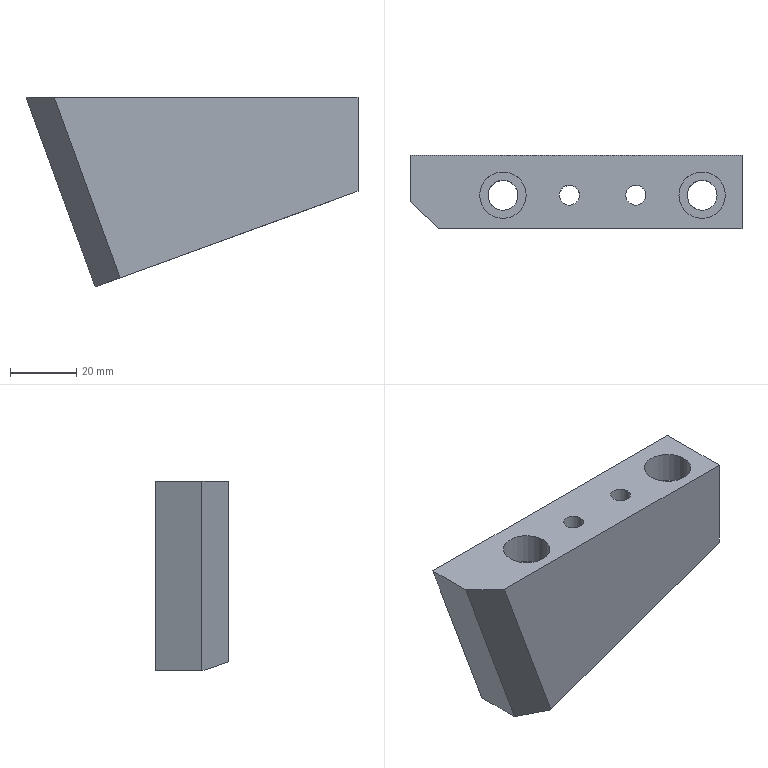Part | STEP file | P011002S003-005 | 1 solid | 15 faces | box 100 x 22 x 57.18 mm | volume 75947 mm3 | plane 9 | cylinder 6 | commonest cylinder face diameters 6 x2 9 x2 14 x2
STEP:
#1=CARTESIAN_POINT('',(0.,0.,0.));
#2=DIRECTION('',(0.,0.,1.));
#3=DIRECTION('',(1.,0.,0.));
#4=AXIS2_PLACEMENT_3D('',#1,#2,#3);
#5=CARTESIAN_POINT('',(-244.,-131.,19.));
#6=VERTEX_POINT('',#5);
#7=CARTESIAN_POINT('',(-237.,-131.,19.));
#8=DIRECTION('',(0.,0.,-1.));
#9=DIRECTION('',(-1.,0.,0.));
#10=AXIS2_PLACEMENT_3D('',#7,#8,#9);
#11=CIRCLE('',#10,7.);
#12=CARTESIAN_POINT('',(-275.,-325.,19.));
#13=DIRECTION('',(0.,0.,1.));
#14=DIRECTION('',(-1.,0.,0.));
#15=AXIS2_PLACEMENT_3D('',#12,#13,#14);
#16=PLANE('',#15);
#17=CARTESIAN_POINT('',(-31.,-194.));
#18=CARTESIAN_POINT('',(-31.,-206.124));
#19=CARTESIAN_POINT('',(-41.5,-200.062));
#20=CARTESIAN_POINT('',(-52.,-194.));
#21=CARTESIAN_POINT('',(-41.5,-187.938));
#22=CARTESIAN_POINT('',(-31.,-181.876));
#23=CARTESIAN_POINT('',(-31.,-194.));
#24=(BOUNDED_CURVE()B_SPLINE_CURVE(2,(#17,#18,#19,#20,#21,#22,#23),.UNSPECIFIED.,.T.,.F.)B_SPLINE_CURVE_WITH_KNOTS((1,2,2,2,2,1),(-2.094,0.,2.094,4.189,6.283,8.378),.UNSPECIFIED.)CURVE()GEOMETRIC_REPRESENTATION_ITEM()RATIONAL_B_SPLINE_CURVE((1.,0.5,1.,0.5,1.,0.5,1.))REPRESENTATION_ITEM(''));
#25=(GEOMETRIC_REPRESENTATION_CONTEXT(2)PARAMETRIC_REPRESENTATION_CONTEXT()REPRESENTATION_CONTEXT('',''));
#26=DEFINITIONAL_REPRESENTATION('',(#24),#25);
#27=PCURVE('',#16,#26);
#28=CARTESIAN_POINT('',(-237.,-131.,19.));
#29=DIRECTION('',(0.,0.,-1.));
#30=DIRECTION('',(1.,0.,0.));
#31=AXIS2_PLACEMENT_3D('',#28,#29,#30);
#32=CYLINDRICAL_SURFACE('',#31,7.);
#33=CARTESIAN_POINT('',(3.142,0.));
#34=DIRECTION('',(1.,0.));
#35=VECTOR('',#34,1.);
#36=LINE('',#33,#35);
#37=(GEOMETRIC_REPRESENTATION_CONTEXT(2)PARAMETRIC_REPRESENTATION_CONTEXT()REPRESENTATION_CONTEXT('',''));
#38=DEFINITIONAL_REPRESENTATION('',(#36),#37);
#39=PCURVE('',#32,#38);
#40=SURFACE_CURVE('',#11,(#27,#39),.PCURVE_S1.);
#41=EDGE_CURVE('',#6,#6,#40,.T.);
#42=ORIENTED_EDGE('',*,*,#41,.T.);
#43=EDGE_LOOP('',(#42));
#44=FACE_BOUND('',#43,.T.);
#45=CARTESIAN_POINT('',(-220.,-131.,19.));
#46=VERTEX_POINT('',#45);
#47=CARTESIAN_POINT('',(-217.,-131.,19.));
#48=DIRECTION('',(0.,0.,-1.));
#49=DIRECTION('',(-1.,0.,0.));
#50=AXIS2_PLACEMENT_3D('',#47,#48,#49);
#51=CIRCLE('',#50,3.);
#52=CARTESIAN_POINT('',(-55.,-194.));
#53=CARTESIAN_POINT('',(-55.,-199.196));
#54=CARTESIAN_POINT('',(-59.5,-196.598));
#55=CARTESIAN_POINT('',(-64.,-194.));
#56=CARTESIAN_POINT('',(-59.5,-191.402));
#57=CARTESIAN_POINT('',(-55.,-188.804));
#58=CARTESIAN_POINT('',(-55.,-194.));
#59=(BOUNDED_CURVE()B_SPLINE_CURVE(2,(#52,#53,#54,#55,#56,#57,#58),.UNSPECIFIED.,.T.,.F.)B_SPLINE_CURVE_WITH_KNOTS((1,2,2,2,2,1),(-2.094,0.,2.094,4.189,6.283,8.378),.UNSPECIFIED.)CURVE()GEOMETRIC_REPRESENTATION_ITEM()RATIONAL_B_SPLINE_CURVE((1.,0.5,1.,0.5,1.,0.5,1.))REPRESENTATION_ITEM(''));
#60=(GEOMETRIC_REPRESENTATION_CONTEXT(2)PARAMETRIC_REPRESENTATION_CONTEXT()REPRESENTATION_CONTEXT('',''));
#61=DEFINITIONAL_REPRESENTATION('',(#59),#60);
#62=PCURVE('',#16,#61);
#63=CARTESIAN_POINT('',(-217.,-131.,19.));
#64=DIRECTION('',(0.,0.,-1.));
#65=DIRECTION('',(1.,0.,0.));
#66=AXIS2_PLACEMENT_3D('',#63,#64,#65);
#67=CYLINDRICAL_SURFACE('',#66,3.);
#68=CARTESIAN_POINT('',(3.142,0.));
#69=DIRECTION('',(1.,0.));
#70=VECTOR('',#69,1.);
#71=LINE('',#68,#70);
#72=(GEOMETRIC_REPRESENTATION_CONTEXT(2)PARAMETRIC_REPRESENTATION_CONTEXT()REPRESENTATION_CONTEXT('',''));
#73=DEFINITIONAL_REPRESENTATION('',(#71),#72);
#74=PCURVE('',#67,#73);
#75=SURFACE_CURVE('',#51,(#62,#74),.PCURVE_S1.);
#76=EDGE_CURVE('',#46,#46,#75,.T.);
#77=ORIENTED_EDGE('',*,*,#76,.T.);
#78=EDGE_LOOP('',(#77));
#79=FACE_BOUND('',#78,.T.);
#80=CARTESIAN_POINT('',(-256.487,-141.,19.));
#81=VERTEX_POINT('',#80);
#82=CARTESIAN_POINT('',(-165.,-141.,19.));
#83=VERTEX_POINT('',#82);
#84=CARTESIAN_POINT('',(-231.38,-141.,19.));
#85=DIRECTION('',(1.,0.,0.));
#86=VECTOR('',#85,1.);
#87=LINE('',#84,#86);
#88=CARTESIAN_POINT('',(-43.62,-184.));
#89=DIRECTION('',(-1.,0.));
#90=VECTOR('',#89,1.);
#91=LINE('',#88,#90);
#92=(GEOMETRIC_REPRESENTATION_CONTEXT(2)PARAMETRIC_REPRESENTATION_CONTEXT()REPRESENTATION_CONTEXT('',''));
#93=DEFINITIONAL_REPRESENTATION('',(#91),#92);
#94=PCURVE('',#16,#93);
#95=CARTESIAN_POINT('',(-231.38,-141.,-33.518));
#96=DIRECTION('',(0.,1.,0.));
#97=DIRECTION('',(0.,0.,1.));
#98=AXIS2_PLACEMENT_3D('',#95,#96,#97);
#99=PLANE('',#98);
#100=CARTESIAN_POINT('',(52.518,0.));
#101=DIRECTION('',(0.,1.));
#102=VECTOR('',#101,1.);
#103=LINE('',#100,#102);
#104=(GEOMETRIC_REPRESENTATION_CONTEXT(2)PARAMETRIC_REPRESENTATION_CONTEXT()REPRESENTATION_CONTEXT('',''));
#105=DEFINITIONAL_REPRESENTATION('',(#103),#104);
#106=PCURVE('',#99,#105);
#107=SURFACE_CURVE('',#87,(#94,#106),.PCURVE_S1.);
#108=EDGE_CURVE('',#81,#83,#107,.T.);
#109=ORIENTED_EDGE('',*,*,#108,.T.);
#110=CARTESIAN_POINT('',(-165.,-119.,19.));
#111=VERTEX_POINT('',#110);
#112=CARTESIAN_POINT('',(-165.,-325.,19.));
#113=DIRECTION('',(0.,-1.,0.));
#114=VECTOR('',#113,1.);
#115=LINE('',#112,#114);
#116=CARTESIAN_POINT('',(-110.,0.));
#117=DIRECTION('',(0.,1.));
#118=VECTOR('',#117,1.);
#119=LINE('',#116,#118);
#120=(GEOMETRIC_REPRESENTATION_CONTEXT(2)PARAMETRIC_REPRESENTATION_CONTEXT()REPRESENTATION_CONTEXT('',''));
#121=DEFINITIONAL_REPRESENTATION('',(#119),#120);
#122=PCURVE('',#16,#121);
#123=CARTESIAN_POINT('',(-165.,-119.,-9.358));
#124=DIRECTION('',(1.,0.,0.));
#125=DIRECTION('',(0.,0.,1.));
#126=AXIS2_PLACEMENT_3D('',#123,#124,#125);
#127=PLANE('',#126);
#128=CARTESIAN_POINT('',(28.358,206.));
#129=DIRECTION('',(0.,1.));
#130=VECTOR('',#129,1.);
#131=LINE('',#128,#130);
#132=(GEOMETRIC_REPRESENTATION_CONTEXT(2)PARAMETRIC_REPRESENTATION_CONTEXT()REPRESENTATION_CONTEXT('',''));
#133=DEFINITIONAL_REPRESENTATION('',(#131),#132);
#134=PCURVE('',#127,#133);
#135=SURFACE_CURVE('',#115,(#122,#134),.PCURVE_S1.);
#136=EDGE_CURVE('',#111,#83,#135,.T.);
#137=ORIENTED_EDGE('',*,*,#136,.F.);
#138=CARTESIAN_POINT('',(-265.,-119.,19.));
#139=VERTEX_POINT('',#138);
#140=CARTESIAN_POINT('',(-231.38,-119.,19.));
#141=DIRECTION('',(1.,0.,0.));
#142=VECTOR('',#141,1.);
#143=LINE('',#140,#142);
#144=CARTESIAN_POINT('',(-43.62,-206.));
#145=DIRECTION('',(-1.,0.));
#146=VECTOR('',#145,1.);
#147=LINE('',#144,#146);
#148=(GEOMETRIC_REPRESENTATION_CONTEXT(2)PARAMETRIC_REPRESENTATION_CONTEXT()REPRESENTATION_CONTEXT('',''));
#149=DEFINITIONAL_REPRESENTATION('',(#147),#148);
#150=PCURVE('',#16,#149);
#151=CARTESIAN_POINT('',(-231.38,-119.,-33.518));
#152=DIRECTION('',(0.,1.,0.));
#153=DIRECTION('',(0.,0.,1.));
#154=AXIS2_PLACEMENT_3D('',#151,#152,#153);
#155=PLANE('',#154);
#156=CARTESIAN_POINT('',(52.518,0.));
#157=DIRECTION('',(0.,1.));
#158=VECTOR('',#157,1.);
#159=LINE('',#156,#158);
#160=(GEOMETRIC_REPRESENTATION_CONTEXT(2)PARAMETRIC_REPRESENTATION_CONTEXT()REPRESENTATION_CONTEXT('',''));
#161=DEFINITIONAL_REPRESENTATION('',(#159),#160);
#162=PCURVE('',#155,#161);
#163=SURFACE_CURVE('',#143,(#150,#162),.PCURVE_S1.);
#164=EDGE_CURVE('',#139,#111,#163,.T.);
#165=ORIENTED_EDGE('',*,*,#164,.F.);
#166=CARTESIAN_POINT('',(-265.,-133.,19.));
#167=VERTEX_POINT('',#166);
#168=CARTESIAN_POINT('',(-265.,-119.,19.));
#169=DIRECTION('',(0.,-1.,0.));
#170=VECTOR('',#169,1.);
#171=LINE('',#168,#170);
#172=CARTESIAN_POINT('',(-10.,-206.));
#173=DIRECTION('',(0.,1.));
#174=VECTOR('',#173,1.);
#175=LINE('',#172,#174);
#176=(GEOMETRIC_REPRESENTATION_CONTEXT(2)PARAMETRIC_REPRESENTATION_CONTEXT()REPRESENTATION_CONTEXT('',''));
#177=DEFINITIONAL_REPRESENTATION('',(#175),#176);
#178=PCURVE('',#16,#177);
#179=CARTESIAN_POINT('',(-265.,-119.,19.));
#180=DIRECTION('',(0.9397,0.,0.342));
#181=DIRECTION('',(-0.342,0.,0.9397));
#182=AXIS2_PLACEMENT_3D('',#179,#180,#181);
#183=PLANE('',#182);
#184=CARTESIAN_POINT('',(0.,0.));
#185=DIRECTION('',(0.,1.));
#186=VECTOR('',#185,1.);
#187=LINE('',#184,#186);
#188=(GEOMETRIC_REPRESENTATION_CONTEXT(2)PARAMETRIC_REPRESENTATION_CONTEXT()REPRESENTATION_CONTEXT('',''));
#189=DEFINITIONAL_REPRESENTATION('',(#187),#188);
#190=PCURVE('',#183,#189);
#191=SURFACE_CURVE('',#171,(#178,#190),.PCURVE_S1.);
#192=EDGE_CURVE('',#139,#167,#191,.T.);
#193=ORIENTED_EDGE('',*,*,#192,.T.);
#194=CARTESIAN_POINT('',(-245.963,-150.889,19.));
#195=DIRECTION('',(-0.7287,0.6848,0.));
#196=VECTOR('',#195,1.);
#197=LINE('',#194,#196);
#198=CARTESIAN_POINT('',(-29.037,-174.111));
#199=DIRECTION('',(0.7287,-0.6848));
#200=VECTOR('',#199,1.);
#201=LINE('',#198,#200);
#202=(GEOMETRIC_REPRESENTATION_CONTEXT(2)PARAMETRIC_REPRESENTATION_CONTEXT()REPRESENTATION_CONTEXT('',''));
#203=DEFINITIONAL_REPRESENTATION('',(#201),#202);
#204=PCURVE('',#16,#203);
#205=CARTESIAN_POINT('',(-236.671,-141.,-35.444));
#206=DIRECTION('',(0.6645,0.7071,0.2418));
#207=DIRECTION('',(0.7287,-0.6848,0.));
#208=AXIS2_PLACEMENT_3D('',#205,#206,#207);
#209=PLANE('',#208);
#210=CARTESIAN_POINT('',(0.,-56.11));
#211=DIRECTION('',(-1.,0.));
#212=VECTOR('',#211,1.);
#213=LINE('',#210,#212);
#214=(GEOMETRIC_REPRESENTATION_CONTEXT(2)PARAMETRIC_REPRESENTATION_CONTEXT()REPRESENTATION_CONTEXT('',''));
#215=DEFINITIONAL_REPRESENTATION('',(#213),#214);
#216=PCURVE('',#209,#215);
#217=SURFACE_CURVE('',#197,(#204,#216),.PCURVE_S1.);
#218=EDGE_CURVE('',#81,#167,#217,.T.);
#219=ORIENTED_EDGE('',*,*,#218,.F.);
#220=EDGE_LOOP('',(#109,#137,#165,#193,#219));
#221=FACE_BOUND('',#220,.T.);
#222=CARTESIAN_POINT('',(-200.,-131.,19.));
#223=VERTEX_POINT('',#222);
#224=CARTESIAN_POINT('',(-197.,-131.,19.));
#225=DIRECTION('',(0.,0.,-1.));
#226=DIRECTION('',(-1.,0.,0.));
#227=AXIS2_PLACEMENT_3D('',#224,#225,#226);
#228=CIRCLE('',#227,3.);
#229=CARTESIAN_POINT('',(-75.,-194.));
#230=CARTESIAN_POINT('',(-75.,-199.196));
#231=CARTESIAN_POINT('',(-79.5,-196.598));
#232=CARTESIAN_POINT('',(-84.,-194.));
#233=CARTESIAN_POINT('',(-79.5,-191.402));
#234=CARTESIAN_POINT('',(-75.,-188.804));
#235=CARTESIAN_POINT('',(-75.,-194.));
#236=(BOUNDED_CURVE()B_SPLINE_CURVE(2,(#229,#230,#231,#232,#233,#234,#235),.UNSPECIFIED.,.T.,.F.)B_SPLINE_CURVE_WITH_KNOTS((1,2,2,2,2,1),(-2.094,0.,2.094,4.189,6.283,8.378),.UNSPECIFIED.)CURVE()GEOMETRIC_REPRESENTATION_ITEM()RATIONAL_B_SPLINE_CURVE((1.,0.5,1.,0.5,1.,0.5,1.))REPRESENTATION_ITEM(''));
#237=(GEOMETRIC_REPRESENTATION_CONTEXT(2)PARAMETRIC_REPRESENTATION_CONTEXT()REPRESENTATION_CONTEXT('',''));
#238=DEFINITIONAL_REPRESENTATION('',(#236),#237);
#239=PCURVE('',#16,#238);
#240=CARTESIAN_POINT('',(-197.,-131.,19.));
#241=DIRECTION('',(0.,0.,-1.));
#242=DIRECTION('',(1.,0.,0.));
#243=AXIS2_PLACEMENT_3D('',#240,#241,#242);
#244=CYLINDRICAL_SURFACE('',#243,3.);
#245=CARTESIAN_POINT('',(3.142,0.));
#246=DIRECTION('',(1.,0.));
#247=VECTOR('',#246,1.);
#248=LINE('',#245,#247);
#249=(GEOMETRIC_REPRESENTATION_CONTEXT(2)PARAMETRIC_REPRESENTATION_CONTEXT()REPRESENTATION_CONTEXT('',''));
#250=DEFINITIONAL_REPRESENTATION('',(#248),#249);
#251=PCURVE('',#244,#250);
#252=SURFACE_CURVE('',#228,(#239,#251),.PCURVE_S1.);
#253=EDGE_CURVE('',#223,#223,#252,.T.);
#254=ORIENTED_EDGE('',*,*,#253,.T.);
#255=EDGE_LOOP('',(#254));
#256=FACE_BOUND('',#255,.T.);
#257=CARTESIAN_POINT('',(-184.,-131.,19.));
#258=VERTEX_POINT('',#257);
#259=CARTESIAN_POINT('',(-177.,-131.,19.));
#260=DIRECTION('',(0.,0.,-1.));
#261=DIRECTION('',(-1.,0.,0.));
#262=AXIS2_PLACEMENT_3D('',#259,#260,#261);
#263=CIRCLE('',#262,7.);
#264=CARTESIAN_POINT('',(-91.,-194.));
#265=CARTESIAN_POINT('',(-91.,-206.124));
#266=CARTESIAN_POINT('',(-101.5,-200.062));
#267=CARTESIAN_POINT('',(-112.,-194.));
#268=CARTESIAN_POINT('',(-101.5,-187.938));
#269=CARTESIAN_POINT('',(-91.,-181.876));
#270=CARTESIAN_POINT('',(-91.,-194.));
#271=(BOUNDED_CURVE()B_SPLINE_CURVE(2,(#264,#265,#266,#267,#268,#269,#270),.UNSPECIFIED.,.T.,.F.)B_SPLINE_CURVE_WITH_KNOTS((1,2,2,2,2,1),(-2.094,0.,2.094,4.189,6.283,8.378),.UNSPECIFIED.)CURVE()GEOMETRIC_REPRESENTATION_ITEM()RATIONAL_B_SPLINE_CURVE((1.,0.5,1.,0.5,1.,0.5,1.))REPRESENTATION_ITEM(''));
#272=(GEOMETRIC_REPRESENTATION_CONTEXT(2)PARAMETRIC_REPRESENTATION_CONTEXT()REPRESENTATION_CONTEXT('',''));
#273=DEFINITIONAL_REPRESENTATION('',(#271),#272);
#274=PCURVE('',#16,#273);
#275=CARTESIAN_POINT('',(-177.,-131.,19.));
#276=DIRECTION('',(0.,0.,-1.));
#277=DIRECTION('',(1.,0.,0.));
#278=AXIS2_PLACEMENT_3D('',#275,#276,#277);
#279=CYLINDRICAL_SURFACE('',#278,7.);
#280=CARTESIAN_POINT('',(3.142,0.));
#281=DIRECTION('',(1.,0.));
#282=VECTOR('',#281,1.);
#283=LINE('',#280,#282);
#284=(GEOMETRIC_REPRESENTATION_CONTEXT(2)PARAMETRIC_REPRESENTATION_CONTEXT()REPRESENTATION_CONTEXT('',''));
#285=DEFINITIONAL_REPRESENTATION('',(#283),#284);
#286=PCURVE('',#279,#285);
#287=SURFACE_CURVE('',#263,(#274,#286),.PCURVE_S1.);
#288=EDGE_CURVE('',#258,#258,#287,.T.);
#289=ORIENTED_EDGE('',*,*,#288,.T.);
#290=EDGE_LOOP('',(#289));
#291=FACE_BOUND('',#290,.T.);
#292=ADVANCED_FACE('',(#44,#79,#221,#256,#291),#16,.T.);
#293=CARTESIAN_POINT('',(-241.5,-131.,-37.202));
#294=VERTEX_POINT('',#293);
#295=CARTESIAN_POINT('',(-237.,-131.,-35.564));
#296=DIRECTION('',(-0.342,0.,0.9397));
#297=DIRECTION('',(-0.9397,0.,-0.342));
#298=AXIS2_PLACEMENT_3D('',#295,#296,#297);
#299=ELLIPSE('',#298,4.789,4.5);
#300=CARTESIAN_POINT('',(-231.38,-119.,-33.518));
#301=DIRECTION('',(0.342,0.,-0.9397));
#302=DIRECTION('',(0.9397,0.,0.342));
#303=AXIS2_PLACEMENT_3D('',#300,#301,#302);
#304=PLANE('',#303);
#305=CARTESIAN_POINT('',(-10.77,12.));
#306=CARTESIAN_POINT('',(-10.77,19.794));
#307=CARTESIAN_POINT('',(-3.587,15.897));
#308=CARTESIAN_POINT('',(3.597,12.));
#309=CARTESIAN_POINT('',(-3.587,8.103));
#310=CARTESIAN_POINT('',(-10.77,4.206));
#311=CARTESIAN_POINT('',(-10.77,12.));
#312=(BOUNDED_CURVE()B_SPLINE_CURVE(2,(#305,#306,#307,#308,#309,#310,#311),.UNSPECIFIED.,.T.,.F.)B_SPLINE_CURVE_WITH_KNOTS((1,2,2,2,2,1),(-2.094,0.,2.094,4.189,6.283,8.378),.UNSPECIFIED.)CURVE()GEOMETRIC_REPRESENTATION_ITEM()RATIONAL_B_SPLINE_CURVE((1.,0.5,1.,0.5,1.,0.5,1.))REPRESENTATION_ITEM(''));
#313=(GEOMETRIC_REPRESENTATION_CONTEXT(2)PARAMETRIC_REPRESENTATION_CONTEXT()REPRESENTATION_CONTEXT('',''));
#314=DEFINITIONAL_REPRESENTATION('',(#312),#313);
#315=PCURVE('',#304,#314);
#316=CARTESIAN_POINT('',(-237.,-131.,19.));
#317=DIRECTION('',(0.,0.,-1.));
#318=DIRECTION('',(1.,0.,0.));
#319=AXIS2_PLACEMENT_3D('',#316,#317,#318);
#320=CYLINDRICAL_SURFACE('',#319,4.5);
#321=CARTESIAN_POINT('',(9.425,56.202));
#322=CARTESIAN_POINT('',(9.33,56.203));
#323=CARTESIAN_POINT('',(9.139,56.157));
#324=CARTESIAN_POINT('',(8.854,55.961));
#325=CARTESIAN_POINT('',(8.568,55.651));
#326=CARTESIAN_POINT('',(8.282,55.254));
#327=CARTESIAN_POINT('',(7.997,54.8));
#328=CARTESIAN_POINT('',(7.711,54.328));
#329=CARTESIAN_POINT('',(7.426,53.874));
#330=CARTESIAN_POINT('',(7.14,53.477));
#331=CARTESIAN_POINT('',(6.854,53.167));
#332=CARTESIAN_POINT('',(6.569,52.971));
#333=CARTESIAN_POINT('',(6.283,52.904));
#334=CARTESIAN_POINT('',(5.998,52.971));
#335=CARTESIAN_POINT('',(5.712,53.167));
#336=CARTESIAN_POINT('',(5.426,53.477));
#337=CARTESIAN_POINT('',(5.141,53.874));
#338=CARTESIAN_POINT('',(4.855,54.328));
#339=CARTESIAN_POINT('',(4.57,54.8));
#340=CARTESIAN_POINT('',(4.284,55.254));
#341=CARTESIAN_POINT('',(3.998,55.651));
#342=CARTESIAN_POINT('',(3.713,55.961));
#343=CARTESIAN_POINT('',(3.427,56.157));
#344=CARTESIAN_POINT('',(3.237,56.203));
#345=CARTESIAN_POINT('',(3.142,56.202));
#346=B_SPLINE_CURVE_WITH_KNOTS('',3,(#321,#322,#323,#324,#325,#326,#327,#328,#329,#330,#331,#332,#333,#334,#335,#336,#337,#338,#339,#340,#341,#342,#343,#344,#345),.UNSPECIFIED.,.F.,.F.,(4,1,1,1,1,1,1,1,1,1,1,1,1,1,1,1,1,1,1,1,1,1,4),(0.,0.2856,0.5712,0.8568,1.142,1.428,1.714,1.999,2.285,2.57,2.856,3.142,3.427,3.713,3.998,4.284,4.57,4.855,5.141,5.426,5.712,5.998,6.283),.QUASI_UNIFORM_KNOTS.);
#347=(GEOMETRIC_REPRESENTATION_CONTEXT(2)PARAMETRIC_REPRESENTATION_CONTEXT()REPRESENTATION_CONTEXT('',''));
#348=DEFINITIONAL_REPRESENTATION('',(#346),#347);
#349=PCURVE('',#320,#348);
#350=SURFACE_CURVE('',#299,(#315,#349),.PCURVE_S1.);
#351=EDGE_CURVE('',#294,#294,#350,.T.);
#352=ORIENTED_EDGE('',*,*,#351,.T.);
#353=EDGE_LOOP('',(#352));
#354=FACE_BOUND('',#353,.T.);
#355=CARTESIAN_POINT('',(-220.,-131.,-29.377));
#356=VERTEX_POINT('',#355);
#357=CARTESIAN_POINT('',(-217.,-131.,-28.285));
#358=DIRECTION('',(-0.342,0.,0.9397));
#359=DIRECTION('',(-0.9397,0.,-0.342));
#360=AXIS2_PLACEMENT_3D('',#357,#358,#359);
#361=ELLIPSE('',#360,3.193,3.);
#362=CARTESIAN_POINT('',(12.11,12.));
#363=CARTESIAN_POINT('',(12.11,17.196));
#364=CARTESIAN_POINT('',(16.899,14.598));
#365=CARTESIAN_POINT('',(21.688,12.));
#366=CARTESIAN_POINT('',(16.899,9.402));
#367=CARTESIAN_POINT('',(12.11,6.804));
#368=CARTESIAN_POINT('',(12.11,12.));
#369=(BOUNDED_CURVE()B_SPLINE_CURVE(2,(#362,#363,#364,#365,#366,#367,#368),.UNSPECIFIED.,.T.,.F.)B_SPLINE_CURVE_WITH_KNOTS((1,2,2,2,2,1),(-2.094,0.,2.094,4.189,6.283,8.378),.UNSPECIFIED.)CURVE()GEOMETRIC_REPRESENTATION_ITEM()RATIONAL_B_SPLINE_CURVE((1.,0.5,1.,0.5,1.,0.5,1.))REPRESENTATION_ITEM(''));
#370=(GEOMETRIC_REPRESENTATION_CONTEXT(2)PARAMETRIC_REPRESENTATION_CONTEXT()REPRESENTATION_CONTEXT('',''));
#371=DEFINITIONAL_REPRESENTATION('',(#369),#370);
#372=PCURVE('',#304,#371);
#373=CARTESIAN_POINT('',(9.425,48.377));
#374=CARTESIAN_POINT('',(9.33,48.377));
#375=CARTESIAN_POINT('',(9.139,48.346));
#376=CARTESIAN_POINT('',(8.854,48.216));
#377=CARTESIAN_POINT('',(8.568,48.009));
#378=CARTESIAN_POINT('',(8.282,47.744));
#379=CARTESIAN_POINT('',(7.997,47.442));
#380=CARTESIAN_POINT('',(7.711,47.127));
#381=CARTESIAN_POINT('',(7.426,46.825));
#382=CARTESIAN_POINT('',(7.14,46.56));
#383=CARTESIAN_POINT('',(6.854,46.354));
#384=CARTESIAN_POINT('',(6.569,46.223));
#385=CARTESIAN_POINT('',(6.283,46.178));
#386=CARTESIAN_POINT('',(5.998,46.223));
#387=CARTESIAN_POINT('',(5.712,46.354));
#388=CARTESIAN_POINT('',(5.426,46.56));
#389=CARTESIAN_POINT('',(5.141,46.825));
#390=CARTESIAN_POINT('',(4.855,47.127));
#391=CARTESIAN_POINT('',(4.57,47.442));
#392=CARTESIAN_POINT('',(4.284,47.744));
#393=CARTESIAN_POINT('',(3.998,48.009));
#394=CARTESIAN_POINT('',(3.713,48.216));
#395=CARTESIAN_POINT('',(3.427,48.346));
#396=CARTESIAN_POINT('',(3.237,48.377));
#397=CARTESIAN_POINT('',(3.142,48.377));
#398=B_SPLINE_CURVE_WITH_KNOTS('',3,(#373,#374,#375,#376,#377,#378,#379,#380,#381,#382,#383,#384,#385,#386,#387,#388,#389,#390,#391,#392,#393,#394,#395,#396,#397),.UNSPECIFIED.,.F.,.F.,(4,1,1,1,1,1,1,1,1,1,1,1,1,1,1,1,1,1,1,1,1,1,4),(0.,0.2856,0.5712,0.8568,1.142,1.428,1.714,1.999,2.285,2.57,2.856,3.142,3.427,3.713,3.998,4.284,4.57,4.855,5.141,5.426,5.712,5.998,6.283),.QUASI_UNIFORM_KNOTS.);
#399=(GEOMETRIC_REPRESENTATION_CONTEXT(2)PARAMETRIC_REPRESENTATION_CONTEXT()REPRESENTATION_CONTEXT('',''));
#400=DEFINITIONAL_REPRESENTATION('',(#398),#399);
#401=PCURVE('',#67,#400);
#402=SURFACE_CURVE('',#361,(#372,#401),.PCURVE_S1.);
#403=EDGE_CURVE('',#356,#356,#402,.T.);
#404=ORIENTED_EDGE('',*,*,#403,.T.);
#405=EDGE_LOOP('',(#404));
#406=FACE_BOUND('',#405,.T.);
#407=CARTESIAN_POINT('',(-244.188,-119.,-38.18));
#408=VERTEX_POINT('',#407);
#409=CARTESIAN_POINT('',(-244.188,-133.,-38.18));
#410=VERTEX_POINT('',#409);
#411=CARTESIAN_POINT('',(-244.188,-119.,-38.18));
#412=DIRECTION('',(0.,-1.,0.));
#413=VECTOR('',#412,1.);
#414=LINE('',#411,#413);
#415=CARTESIAN_POINT('',(-13.63,0.));
#416=DIRECTION('',(0.,1.));
#417=VECTOR('',#416,1.);
#418=LINE('',#415,#417);
#419=(GEOMETRIC_REPRESENTATION_CONTEXT(2)PARAMETRIC_REPRESENTATION_CONTEXT()REPRESENTATION_CONTEXT('',''));
#420=DEFINITIONAL_REPRESENTATION('',(#418),#419);
#421=PCURVE('',#304,#420);
#422=CARTESIAN_POINT('',(-60.85,0.));
#423=DIRECTION('',(0.,1.));
#424=VECTOR('',#423,1.);
#425=LINE('',#422,#424);
#426=(GEOMETRIC_REPRESENTATION_CONTEXT(2)PARAMETRIC_REPRESENTATION_CONTEXT()REPRESENTATION_CONTEXT('',''));
#427=DEFINITIONAL_REPRESENTATION('',(#425),#426);
#428=PCURVE('',#183,#427);
#429=SURFACE_CURVE('',#414,(#421,#428),.PCURVE_S1.);
#430=EDGE_CURVE('',#408,#410,#429,.T.);
#431=ORIENTED_EDGE('',*,*,#430,.F.);
#432=CARTESIAN_POINT('',(-165.,-119.,-9.358));
#433=VERTEX_POINT('',#432);
#434=CARTESIAN_POINT('',(-231.38,-119.,-33.518));
#435=DIRECTION('',(0.9397,0.,0.342));
#436=VECTOR('',#435,1.);
#437=LINE('',#434,#436);
#438=CARTESIAN_POINT('',(0.,0.));
#439=DIRECTION('',(1.,0.));
#440=VECTOR('',#439,1.);
#441=LINE('',#438,#440);
#442=(GEOMETRIC_REPRESENTATION_CONTEXT(2)PARAMETRIC_REPRESENTATION_CONTEXT()REPRESENTATION_CONTEXT('',''));
#443=DEFINITIONAL_REPRESENTATION('',(#441),#442);
#444=PCURVE('',#304,#443);
#445=CARTESIAN_POINT('',(0.,0.));
#446=DIRECTION('',(0.342,0.9397));
#447=VECTOR('',#446,1.);
#448=LINE('',#445,#447);
#449=(GEOMETRIC_REPRESENTATION_CONTEXT(2)PARAMETRIC_REPRESENTATION_CONTEXT()REPRESENTATION_CONTEXT('',''));
#450=DEFINITIONAL_REPRESENTATION('',(#448),#449);
#451=PCURVE('',#155,#450);
#452=SURFACE_CURVE('',#437,(#444,#451),.PCURVE_S1.);
#453=EDGE_CURVE('',#408,#433,#452,.T.);
#454=ORIENTED_EDGE('',*,*,#453,.T.);
#455=CARTESIAN_POINT('',(-165.,-141.,-9.358));
#456=VERTEX_POINT('',#455);
#457=CARTESIAN_POINT('',(-165.,-119.,-9.358));
#458=DIRECTION('',(0.,-1.,0.));
#459=VECTOR('',#458,1.);
#460=LINE('',#457,#459);
#461=CARTESIAN_POINT('',(70.64,0.));
#462=DIRECTION('',(0.,1.));
#463=VECTOR('',#462,1.);
#464=LINE('',#461,#463);
#465=(GEOMETRIC_REPRESENTATION_CONTEXT(2)PARAMETRIC_REPRESENTATION_CONTEXT()REPRESENTATION_CONTEXT('',''));
#466=DEFINITIONAL_REPRESENTATION('',(#464),#465);
#467=PCURVE('',#304,#466);
#468=CARTESIAN_POINT('',(0.,0.));
#469=DIRECTION('',(0.,1.));
#470=VECTOR('',#469,1.);
#471=LINE('',#468,#470);
#472=(GEOMETRIC_REPRESENTATION_CONTEXT(2)PARAMETRIC_REPRESENTATION_CONTEXT()REPRESENTATION_CONTEXT('',''));
#473=DEFINITIONAL_REPRESENTATION('',(#471),#472);
#474=PCURVE('',#127,#473);
#475=SURFACE_CURVE('',#460,(#467,#474),.PCURVE_S1.);
#476=EDGE_CURVE('',#433,#456,#475,.T.);
#477=ORIENTED_EDGE('',*,*,#476,.T.);
#478=CARTESIAN_POINT('',(-236.671,-141.,-35.444));
#479=VERTEX_POINT('',#478);
#480=CARTESIAN_POINT('',(-231.38,-141.,-33.518));
#481=DIRECTION('',(0.9397,0.,0.342));
#482=VECTOR('',#481,1.);
#483=LINE('',#480,#482);
#484=CARTESIAN_POINT('',(0.,22.));
#485=DIRECTION('',(1.,0.));
#486=VECTOR('',#485,1.);
#487=LINE('',#484,#486);
#488=(GEOMETRIC_REPRESENTATION_CONTEXT(2)PARAMETRIC_REPRESENTATION_CONTEXT()REPRESENTATION_CONTEXT('',''));
#489=DEFINITIONAL_REPRESENTATION('',(#487),#488);
#490=PCURVE('',#304,#489);
#491=CARTESIAN_POINT('',(0.,0.));
#492=DIRECTION('',(0.342,0.9397));
#493=VECTOR('',#492,1.);
#494=LINE('',#491,#493);
#495=(GEOMETRIC_REPRESENTATION_CONTEXT(2)PARAMETRIC_REPRESENTATION_CONTEXT()REPRESENTATION_CONTEXT('',''));
#496=DEFINITIONAL_REPRESENTATION('',(#494),#495);
#497=PCURVE('',#99,#496);
#498=SURFACE_CURVE('',#483,(#490,#497),.PCURVE_S1.);
#499=EDGE_CURVE('',#479,#456,#498,.T.);
#500=ORIENTED_EDGE('',*,*,#499,.F.);
#501=CARTESIAN_POINT('',(-236.671,-141.,-35.444));
#502=DIRECTION('',(0.6645,-0.7071,0.2418));
#503=VECTOR('',#502,1.);
#504=LINE('',#501,#503);
#505=CARTESIAN_POINT('',(-5.63,22.));
#506=DIRECTION('',(0.7071,0.7071));
#507=VECTOR('',#506,1.);
#508=LINE('',#505,#507);
#509=(GEOMETRIC_REPRESENTATION_CONTEXT(2)PARAMETRIC_REPRESENTATION_CONTEXT()REPRESENTATION_CONTEXT('',''));
#510=DEFINITIONAL_REPRESENTATION('',(#508),#509);
#511=PCURVE('',#304,#510);
#512=CARTESIAN_POINT('',(0.,0.));
#513=DIRECTION('',(0.9684,-0.2492));
#514=VECTOR('',#513,1.);
#515=LINE('',#512,#514);
#516=(GEOMETRIC_REPRESENTATION_CONTEXT(2)PARAMETRIC_REPRESENTATION_CONTEXT()REPRESENTATION_CONTEXT('',''));
#517=DEFINITIONAL_REPRESENTATION('',(#515),#516);
#518=PCURVE('',#209,#517);
#519=SURFACE_CURVE('',#504,(#511,#518),.PCURVE_S1.);
#520=EDGE_CURVE('',#410,#479,#519,.T.);
#521=ORIENTED_EDGE('',*,*,#520,.F.);
#522=EDGE_LOOP('',(#431,#454,#477,#500,#521));
#523=FACE_BOUND('',#522,.T.);
#524=CARTESIAN_POINT('',(-200.,-131.,-22.097));
#525=VERTEX_POINT('',#524);
#526=CARTESIAN_POINT('',(-197.,-131.,-21.005));
#527=DIRECTION('',(-0.342,0.,0.9397));
#528=DIRECTION('',(-0.9397,0.,-0.342));
#529=AXIS2_PLACEMENT_3D('',#526,#527,#528);
#530=ELLIPSE('',#529,3.193,3.);
#531=CARTESIAN_POINT('',(33.393,12.));
#532=CARTESIAN_POINT('',(33.393,17.196));
#533=CARTESIAN_POINT('',(38.182,14.598));
#534=CARTESIAN_POINT('',(42.971,12.));
#535=CARTESIAN_POINT('',(38.182,9.402));
#536=CARTESIAN_POINT('',(33.393,6.804));
#537=CARTESIAN_POINT('',(33.393,12.));
#538=(BOUNDED_CURVE()B_SPLINE_CURVE(2,(#531,#532,#533,#534,#535,#536,#537),.UNSPECIFIED.,.T.,.F.)B_SPLINE_CURVE_WITH_KNOTS((1,2,2,2,2,1),(-2.094,0.,2.094,4.189,6.283,8.378),.UNSPECIFIED.)CURVE()GEOMETRIC_REPRESENTATION_ITEM()RATIONAL_B_SPLINE_CURVE((1.,0.5,1.,0.5,1.,0.5,1.))REPRESENTATION_ITEM(''));
#539=(GEOMETRIC_REPRESENTATION_CONTEXT(2)PARAMETRIC_REPRESENTATION_CONTEXT()REPRESENTATION_CONTEXT('',''));
#540=DEFINITIONAL_REPRESENTATION('',(#538),#539);
#541=PCURVE('',#304,#540);
#542=CARTESIAN_POINT('',(9.425,41.097));
#543=CARTESIAN_POINT('',(9.33,41.098));
#544=CARTESIAN_POINT('',(9.139,41.067));
#545=CARTESIAN_POINT('',(8.854,40.936));
#546=CARTESIAN_POINT('',(8.568,40.73));
#547=CARTESIAN_POINT('',(8.282,40.465));
#548=CARTESIAN_POINT('',(7.997,40.163));
#549=CARTESIAN_POINT('',(7.711,39.848));
#550=CARTESIAN_POINT('',(7.426,39.545));
#551=CARTESIAN_POINT('',(7.14,39.28));
#552=CARTESIAN_POINT('',(6.854,39.074));
#553=CARTESIAN_POINT('',(6.569,38.943));
#554=CARTESIAN_POINT('',(6.283,38.898));
#555=CARTESIAN_POINT('',(5.998,38.943));
#556=CARTESIAN_POINT('',(5.712,39.074));
#557=CARTESIAN_POINT('',(5.426,39.28));
#558=CARTESIAN_POINT('',(5.141,39.545));
#559=CARTESIAN_POINT('',(4.855,39.848));
#560=CARTESIAN_POINT('',(4.57,40.163));
#561=CARTESIAN_POINT('',(4.284,40.465));
#562=CARTESIAN_POINT('',(3.998,40.73));
#563=CARTESIAN_POINT('',(3.713,40.936));
#564=CARTESIAN_POINT('',(3.427,41.067));
#565=CARTESIAN_POINT('',(3.237,41.098));
#566=CARTESIAN_POINT('',(3.142,41.097));
#567=B_SPLINE_CURVE_WITH_KNOTS('',3,(#542,#543,#544,#545,#546,#547,#548,#549,#550,#551,#552,#553,#554,#555,#556,#557,#558,#559,#560,#561,#562,#563,#564,#565,#566),.UNSPECIFIED.,.F.,.F.,(4,1,1,1,1,1,1,1,1,1,1,1,1,1,1,1,1,1,1,1,1,1,4),(0.,0.2856,0.5712,0.8568,1.142,1.428,1.714,1.999,2.285,2.57,2.856,3.142,3.427,3.713,3.998,4.284,4.57,4.855,5.141,5.426,5.712,5.998,6.283),.QUASI_UNIFORM_KNOTS.);
#568=(GEOMETRIC_REPRESENTATION_CONTEXT(2)PARAMETRIC_REPRESENTATION_CONTEXT()REPRESENTATION_CONTEXT('',''));
#569=DEFINITIONAL_REPRESENTATION('',(#567),#568);
#570=PCURVE('',#244,#569);
#571=SURFACE_CURVE('',#530,(#541,#570),.PCURVE_S1.);
#572=EDGE_CURVE('',#525,#525,#571,.T.);
#573=ORIENTED_EDGE('',*,*,#572,.T.);
#574=EDGE_LOOP('',(#573));
#575=FACE_BOUND('',#574,.T.);
#576=CARTESIAN_POINT('',(-181.5,-131.,-15.364));
#577=VERTEX_POINT('',#576);
#578=CARTESIAN_POINT('',(-177.,-131.,-13.726));
#579=DIRECTION('',(-0.342,0.,0.9397));
#580=DIRECTION('',(-0.9397,0.,-0.342));
#581=AXIS2_PLACEMENT_3D('',#578,#579,#580);
#582=ELLIPSE('',#581,4.789,4.5);
#583=CARTESIAN_POINT('',(53.081,12.));
#584=CARTESIAN_POINT('',(53.081,19.794));
#585=CARTESIAN_POINT('',(60.264,15.897));
#586=CARTESIAN_POINT('',(67.447,12.));
#587=CARTESIAN_POINT('',(60.264,8.103));
#588=CARTESIAN_POINT('',(53.081,4.206));
#589=CARTESIAN_POINT('',(53.081,12.));
#590=(BOUNDED_CURVE()B_SPLINE_CURVE(2,(#583,#584,#585,#586,#587,#588,#589),.UNSPECIFIED.,.T.,.F.)B_SPLINE_CURVE_WITH_KNOTS((1,2,2,2,2,1),(-2.094,0.,2.094,4.189,6.283,8.378),.UNSPECIFIED.)CURVE()GEOMETRIC_REPRESENTATION_ITEM()RATIONAL_B_SPLINE_CURVE((1.,0.5,1.,0.5,1.,0.5,1.))REPRESENTATION_ITEM(''));
#591=(GEOMETRIC_REPRESENTATION_CONTEXT(2)PARAMETRIC_REPRESENTATION_CONTEXT()REPRESENTATION_CONTEXT('',''));
#592=DEFINITIONAL_REPRESENTATION('',(#590),#591);
#593=PCURVE('',#304,#592);
#594=CARTESIAN_POINT('',(-177.,-131.,19.));
#595=DIRECTION('',(0.,0.,-1.));
#596=DIRECTION('',(1.,0.,0.));
#597=AXIS2_PLACEMENT_3D('',#594,#595,#596);
#598=CYLINDRICAL_SURFACE('',#597,4.5);
#599=CARTESIAN_POINT('',(9.425,34.364));
#600=CARTESIAN_POINT('',(9.33,34.365));
#601=CARTESIAN_POINT('',(9.139,34.319));
#602=CARTESIAN_POINT('',(8.854,34.123));
#603=CARTESIAN_POINT('',(8.568,33.813));
#604=CARTESIAN_POINT('',(8.282,33.416));
#605=CARTESIAN_POINT('',(7.997,32.962));
#606=CARTESIAN_POINT('',(7.711,32.49));
#607=CARTESIAN_POINT('',(7.426,32.036));
#608=CARTESIAN_POINT('',(7.14,31.639));
#609=CARTESIAN_POINT('',(6.854,31.329));
#610=CARTESIAN_POINT('',(6.569,31.133));
#611=CARTESIAN_POINT('',(6.283,31.066));
#612=CARTESIAN_POINT('',(5.998,31.133));
#613=CARTESIAN_POINT('',(5.712,31.329));
#614=CARTESIAN_POINT('',(5.426,31.639));
#615=CARTESIAN_POINT('',(5.141,32.036));
#616=CARTESIAN_POINT('',(4.855,32.49));
#617=CARTESIAN_POINT('',(4.57,32.962));
#618=CARTESIAN_POINT('',(4.284,33.416));
#619=CARTESIAN_POINT('',(3.998,33.813));
#620=CARTESIAN_POINT('',(3.713,34.123));
#621=CARTESIAN_POINT('',(3.427,34.319));
#622=CARTESIAN_POINT('',(3.237,34.365));
#623=CARTESIAN_POINT('',(3.142,34.364));
#624=B_SPLINE_CURVE_WITH_KNOTS('',3,(#599,#600,#601,#602,#603,#604,#605,#606,#607,#608,#609,#610,#611,#612,#613,#614,#615,#616,#617,#618,#619,#620,#621,#622,#623),.UNSPECIFIED.,.F.,.F.,(4,1,1,1,1,1,1,1,1,1,1,1,1,1,1,1,1,1,1,1,1,1,4),(0.,0.2856,0.5712,0.8568,1.142,1.428,1.714,1.999,2.285,2.57,2.856,3.142,3.427,3.713,3.998,4.284,4.57,4.855,5.141,5.426,5.712,5.998,6.283),.QUASI_UNIFORM_KNOTS.);
#625=(GEOMETRIC_REPRESENTATION_CONTEXT(2)PARAMETRIC_REPRESENTATION_CONTEXT()REPRESENTATION_CONTEXT('',''));
#626=DEFINITIONAL_REPRESENTATION('',(#624),#625);
#627=PCURVE('',#598,#626);
#628=SURFACE_CURVE('',#582,(#593,#627),.PCURVE_S1.);
#629=EDGE_CURVE('',#577,#577,#628,.T.);
#630=ORIENTED_EDGE('',*,*,#629,.T.);
#631=EDGE_LOOP('',(#630));
#632=FACE_BOUND('',#631,.T.);
#633=ADVANCED_FACE('',(#354,#406,#523,#575,#632),#304,.T.);
#634=ORIENTED_EDGE('',*,*,#476,.F.);
#635=CARTESIAN_POINT('',(-165.,-119.,-9.358));
#636=DIRECTION('',(0.,0.,1.));
#637=VECTOR('',#636,1.);
#638=LINE('',#635,#637);
#639=CARTESIAN_POINT('',(0.,0.));
#640=DIRECTION('',(1.,0.));
#641=VECTOR('',#640,1.);
#642=LINE('',#639,#641);
#643=(GEOMETRIC_REPRESENTATION_CONTEXT(2)PARAMETRIC_REPRESENTATION_CONTEXT()REPRESENTATION_CONTEXT('',''));
#644=DEFINITIONAL_REPRESENTATION('',(#642),#643);
#645=PCURVE('',#127,#644);
#646=CARTESIAN_POINT('',(24.16,66.38));
#647=DIRECTION('',(1.,0.));
#648=VECTOR('',#647,1.);
#649=LINE('',#646,#648);
#650=(GEOMETRIC_REPRESENTATION_CONTEXT(2)PARAMETRIC_REPRESENTATION_CONTEXT()REPRESENTATION_CONTEXT('',''));
#651=DEFINITIONAL_REPRESENTATION('',(#649),#650);
#652=PCURVE('',#155,#651);
#653=SURFACE_CURVE('',#638,(#645,#652),.PCURVE_S1.);
#654=EDGE_CURVE('',#433,#111,#653,.T.);
#655=ORIENTED_EDGE('',*,*,#654,.T.);
#656=ORIENTED_EDGE('',*,*,#136,.T.);
#657=CARTESIAN_POINT('',(-165.,-141.,-9.358));
#658=DIRECTION('',(0.,0.,1.));
#659=VECTOR('',#658,1.);
#660=LINE('',#657,#659);
#661=CARTESIAN_POINT('',(0.,22.));
#662=DIRECTION('',(1.,0.));
#663=VECTOR('',#662,1.);
#664=LINE('',#661,#663);
#665=(GEOMETRIC_REPRESENTATION_CONTEXT(2)PARAMETRIC_REPRESENTATION_CONTEXT()REPRESENTATION_CONTEXT('',''));
#666=DEFINITIONAL_REPRESENTATION('',(#664),#665);
#667=PCURVE('',#127,#666);
#668=CARTESIAN_POINT('',(24.16,66.38));
#669=DIRECTION('',(1.,0.));
#670=VECTOR('',#669,1.);
#671=LINE('',#668,#670);
#672=(GEOMETRIC_REPRESENTATION_CONTEXT(2)PARAMETRIC_REPRESENTATION_CONTEXT()REPRESENTATION_CONTEXT('',''));
#673=DEFINITIONAL_REPRESENTATION('',(#671),#672);
#674=PCURVE('',#99,#673);
#675=SURFACE_CURVE('',#660,(#667,#674),.PCURVE_S1.);
#676=EDGE_CURVE('',#456,#83,#675,.T.);
#677=ORIENTED_EDGE('',*,*,#676,.F.);
#678=EDGE_LOOP('',(#634,#655,#656,#677));
#679=FACE_BOUND('',#678,.T.);
#680=ADVANCED_FACE('',(#679),#127,.T.);
#681=ORIENTED_EDGE('',*,*,#192,.F.);
#682=CARTESIAN_POINT('',(-244.188,-119.,-38.18));
#683=DIRECTION('',(-0.342,0.,0.9397));
#684=VECTOR('',#683,1.);
#685=LINE('',#682,#684);
#686=CARTESIAN_POINT('',(-60.85,0.));
#687=DIRECTION('',(1.,0.));
#688=VECTOR('',#687,1.);
#689=LINE('',#686,#688);
#690=(GEOMETRIC_REPRESENTATION_CONTEXT(2)PARAMETRIC_REPRESENTATION_CONTEXT()REPRESENTATION_CONTEXT('',''));
#691=DEFINITIONAL_REPRESENTATION('',(#689),#690);
#692=PCURVE('',#183,#691);
#693=CARTESIAN_POINT('',(-4.662,-12.808));
#694=DIRECTION('',(0.9397,-0.342));
#695=VECTOR('',#694,1.);
#696=LINE('',#693,#695);
#697=(GEOMETRIC_REPRESENTATION_CONTEXT(2)PARAMETRIC_REPRESENTATION_CONTEXT()REPRESENTATION_CONTEXT('',''));
#698=DEFINITIONAL_REPRESENTATION('',(#696),#697);
#699=PCURVE('',#155,#698);
#700=SURFACE_CURVE('',#685,(#692,#699),.PCURVE_S1.);
#701=EDGE_CURVE('',#408,#139,#700,.T.);
#702=ORIENTED_EDGE('',*,*,#701,.F.);
#703=ORIENTED_EDGE('',*,*,#430,.T.);
#704=CARTESIAN_POINT('',(-265.,-133.,19.));
#705=DIRECTION('',(0.342,0.,-0.9397));
#706=VECTOR('',#705,1.);
#707=LINE('',#704,#706);
#708=CARTESIAN_POINT('',(0.,14.));
#709=DIRECTION('',(-1.,0.));
#710=VECTOR('',#709,1.);
#711=LINE('',#708,#710);
#712=(GEOMETRIC_REPRESENTATION_CONTEXT(2)PARAMETRIC_REPRESENTATION_CONTEXT()REPRESENTATION_CONTEXT('',''));
#713=DEFINITIONAL_REPRESENTATION('',(#711),#712);
#714=PCURVE('',#183,#713);
#715=CARTESIAN_POINT('',(-26.123,-56.11));
#716=DIRECTION('',(0.2492,0.9684));
#717=VECTOR('',#716,1.);
#718=LINE('',#715,#717);
#719=(GEOMETRIC_REPRESENTATION_CONTEXT(2)PARAMETRIC_REPRESENTATION_CONTEXT()REPRESENTATION_CONTEXT('',''));
#720=DEFINITIONAL_REPRESENTATION('',(#718),#719);
#721=PCURVE('',#209,#720);
#722=SURFACE_CURVE('',#707,(#714,#721),.PCURVE_S1.);
#723=EDGE_CURVE('',#167,#410,#722,.T.);
#724=ORIENTED_EDGE('',*,*,#723,.F.);
#725=EDGE_LOOP('',(#681,#702,#703,#724));
#726=FACE_BOUND('',#725,.T.);
#727=ADVANCED_FACE('',(#726),#183,.F.);
#728=ORIENTED_EDGE('',*,*,#499,.T.);
#729=ORIENTED_EDGE('',*,*,#676,.T.);
#730=ORIENTED_EDGE('',*,*,#108,.F.);
#731=CARTESIAN_POINT('',(-236.671,-141.,-35.444));
#732=DIRECTION('',(-0.342,0.,0.9397));
#733=VECTOR('',#732,1.);
#734=LINE('',#731,#733);
#735=CARTESIAN_POINT('',(-1.926,-5.291));
#736=DIRECTION('',(0.9397,-0.342));
#737=VECTOR('',#736,1.);
#738=LINE('',#735,#737);
#739=(GEOMETRIC_REPRESENTATION_CONTEXT(2)PARAMETRIC_REPRESENTATION_CONTEXT()REPRESENTATION_CONTEXT('',''));
#740=DEFINITIONAL_REPRESENTATION('',(#738),#739);
#741=PCURVE('',#99,#740);
#742=CARTESIAN_POINT('',(0.,0.));
#743=DIRECTION('',(-0.2492,-0.9684));
#744=VECTOR('',#743,1.);
#745=LINE('',#742,#744);
#746=(GEOMETRIC_REPRESENTATION_CONTEXT(2)PARAMETRIC_REPRESENTATION_CONTEXT()REPRESENTATION_CONTEXT('',''));
#747=DEFINITIONAL_REPRESENTATION('',(#745),#746);
#748=PCURVE('',#209,#747);
#749=SURFACE_CURVE('',#734,(#741,#748),.PCURVE_S1.);
#750=EDGE_CURVE('',#479,#81,#749,.T.);
#751=ORIENTED_EDGE('',*,*,#750,.F.);
#752=EDGE_LOOP('',(#728,#729,#730,#751));
#753=FACE_BOUND('',#752,.T.);
#754=ADVANCED_FACE('',(#753),#99,.F.);
#755=ORIENTED_EDGE('',*,*,#164,.T.);
#756=ORIENTED_EDGE('',*,*,#654,.F.);
#757=ORIENTED_EDGE('',*,*,#453,.F.);
#758=ORIENTED_EDGE('',*,*,#701,.T.);
#759=EDGE_LOOP('',(#755,#756,#757,#758));
#760=FACE_BOUND('',#759,.T.);
#761=ADVANCED_FACE('',(#760),#155,.T.);
#762=ORIENTED_EDGE('',*,*,#520,.T.);
#763=ORIENTED_EDGE('',*,*,#750,.T.);
#764=ORIENTED_EDGE('',*,*,#218,.T.);
#765=ORIENTED_EDGE('',*,*,#723,.T.);
#766=EDGE_LOOP('',(#762,#763,#764,#765));
#767=FACE_BOUND('',#766,.T.);
#768=ADVANCED_FACE('',(#767),#209,.F.);
#769=ORIENTED_EDGE('',*,*,#76,.T.);
#770=CARTESIAN_POINT('',(-220.,-131.,19.));
#771=CARTESIAN_POINT('',(-220.,-131.,-29.377));
#772=B_SPLINE_CURVE_WITH_KNOTS('',1,(#770,#771),.UNSPECIFIED.,.F.,.F.,(2,2),(0.,48.377),.PIECEWISE_BEZIER_KNOTS.);
#773=CARTESIAN_POINT('',(9.425,0.));
#774=DIRECTION('',(0.,1.));
#775=VECTOR('',#774,1.);
#776=LINE('',#773,#775);
#777=(GEOMETRIC_REPRESENTATION_CONTEXT(2)PARAMETRIC_REPRESENTATION_CONTEXT()REPRESENTATION_CONTEXT('',''));
#778=DEFINITIONAL_REPRESENTATION('',(#776),#777);
#779=PCURVE('',#67,#778);
#780=CARTESIAN_POINT('',(3.142,0.));
#781=DIRECTION('',(0.,1.));
#782=VECTOR('',#781,1.);
#783=LINE('',#780,#782);
#784=(GEOMETRIC_REPRESENTATION_CONTEXT(2)PARAMETRIC_REPRESENTATION_CONTEXT()REPRESENTATION_CONTEXT('',''));
#785=DEFINITIONAL_REPRESENTATION('',(#783),#784);
#786=PCURVE('',#67,#785);
#787=SEAM_CURVE('',#772,(#779,#786),.PCURVE_S1.);
#788=EDGE_CURVE('',#46,#356,#787,.T.);
#789=ORIENTED_EDGE('',*,*,#788,.T.);
#790=ORIENTED_EDGE('',*,*,#403,.T.);
#791=ORIENTED_EDGE('',*,*,#788,.F.);
#792=EDGE_LOOP('',(#769,#789,#790,#791));
#793=FACE_BOUND('',#792,.F.);
#794=ADVANCED_FACE('',(#793),#67,.F.);
#795=ORIENTED_EDGE('',*,*,#253,.T.);
#796=CARTESIAN_POINT('',(-200.,-131.,19.));
#797=CARTESIAN_POINT('',(-200.,-131.,-22.097));
#798=B_SPLINE_CURVE_WITH_KNOTS('',1,(#796,#797),.UNSPECIFIED.,.F.,.F.,(2,2),(0.,41.097),.PIECEWISE_BEZIER_KNOTS.);
#799=CARTESIAN_POINT('',(9.425,0.));
#800=DIRECTION('',(0.,1.));
#801=VECTOR('',#800,1.);
#802=LINE('',#799,#801);
#803=(GEOMETRIC_REPRESENTATION_CONTEXT(2)PARAMETRIC_REPRESENTATION_CONTEXT()REPRESENTATION_CONTEXT('',''));
#804=DEFINITIONAL_REPRESENTATION('',(#802),#803);
#805=PCURVE('',#244,#804);
#806=CARTESIAN_POINT('',(3.142,0.));
#807=DIRECTION('',(0.,1.));
#808=VECTOR('',#807,1.);
#809=LINE('',#806,#808);
#810=(GEOMETRIC_REPRESENTATION_CONTEXT(2)PARAMETRIC_REPRESENTATION_CONTEXT()REPRESENTATION_CONTEXT('',''));
#811=DEFINITIONAL_REPRESENTATION('',(#809),#810);
#812=PCURVE('',#244,#811);
#813=SEAM_CURVE('',#798,(#805,#812),.PCURVE_S1.);
#814=EDGE_CURVE('',#223,#525,#813,.T.);
#815=ORIENTED_EDGE('',*,*,#814,.T.);
#816=ORIENTED_EDGE('',*,*,#572,.T.);
#817=ORIENTED_EDGE('',*,*,#814,.F.);
#818=EDGE_LOOP('',(#795,#815,#816,#817));
#819=FACE_BOUND('',#818,.F.);
#820=ADVANCED_FACE('',(#819),#244,.F.);
#821=CARTESIAN_POINT('',(-241.5,-131.,9.5));
#822=VERTEX_POINT('',#821);
#823=CARTESIAN_POINT('',(-237.,-131.,9.5));
#824=DIRECTION('',(0.,0.,-1.));
#825=DIRECTION('',(-1.,0.,0.));
#826=AXIS2_PLACEMENT_3D('',#823,#824,#825);
#827=CIRCLE('',#826,4.5);
#828=CARTESIAN_POINT('',(3.142,9.5));
#829=DIRECTION('',(1.,0.));
#830=VECTOR('',#829,1.);
#831=LINE('',#828,#830);
#832=(GEOMETRIC_REPRESENTATION_CONTEXT(2)PARAMETRIC_REPRESENTATION_CONTEXT()REPRESENTATION_CONTEXT('',''));
#833=DEFINITIONAL_REPRESENTATION('',(#831),#832);
#834=PCURVE('',#320,#833);
#835=CARTESIAN_POINT('',(-215.,112.,9.5));
#836=DIRECTION('',(0.,0.,1.));
#837=DIRECTION('',(-1.,0.,0.));
#838=AXIS2_PLACEMENT_3D('',#835,#836,#837);
#839=PLANE('',#838);
#840=CARTESIAN_POINT('',(26.5,243.));
#841=CARTESIAN_POINT('',(26.5,235.206));
#842=CARTESIAN_POINT('',(19.75,239.103));
#843=CARTESIAN_POINT('',(13.,243.));
#844=CARTESIAN_POINT('',(19.75,246.897));
#845=CARTESIAN_POINT('',(26.5,250.794));
#846=CARTESIAN_POINT('',(26.5,243.));
#847=(BOUNDED_CURVE()B_SPLINE_CURVE(2,(#840,#841,#842,#843,#844,#845,#846),.UNSPECIFIED.,.T.,.F.)B_SPLINE_CURVE_WITH_KNOTS((1,2,2,2,2,1),(-2.094,0.,2.094,4.189,6.283,8.378),.UNSPECIFIED.)CURVE()GEOMETRIC_REPRESENTATION_ITEM()RATIONAL_B_SPLINE_CURVE((1.,0.5,1.,0.5,1.,0.5,1.))REPRESENTATION_ITEM(''));
#848=(GEOMETRIC_REPRESENTATION_CONTEXT(2)PARAMETRIC_REPRESENTATION_CONTEXT()REPRESENTATION_CONTEXT('',''));
#849=DEFINITIONAL_REPRESENTATION('',(#847),#848);
#850=PCURVE('',#839,#849);
#851=SURFACE_CURVE('',#827,(#834,#850),.PCURVE_S1.);
#852=EDGE_CURVE('',#822,#822,#851,.T.);
#853=ORIENTED_EDGE('',*,*,#852,.T.);
#854=CARTESIAN_POINT('',(-241.5,-131.,9.5));
#855=CARTESIAN_POINT('',(-241.5,-131.,-37.202));
#856=B_SPLINE_CURVE_WITH_KNOTS('',1,(#854,#855),.UNSPECIFIED.,.F.,.F.,(2,2),(9.5,56.202),.PIECEWISE_BEZIER_KNOTS.);
#857=CARTESIAN_POINT('',(9.425,0.));
#858=DIRECTION('',(0.,1.));
#859=VECTOR('',#858,1.);
#860=LINE('',#857,#859);
#861=(GEOMETRIC_REPRESENTATION_CONTEXT(2)PARAMETRIC_REPRESENTATION_CONTEXT()REPRESENTATION_CONTEXT('',''));
#862=DEFINITIONAL_REPRESENTATION('',(#860),#861);
#863=PCURVE('',#320,#862);
#864=CARTESIAN_POINT('',(3.142,0.));
#865=DIRECTION('',(0.,1.));
#866=VECTOR('',#865,1.);
#867=LINE('',#864,#866);
#868=(GEOMETRIC_REPRESENTATION_CONTEXT(2)PARAMETRIC_REPRESENTATION_CONTEXT()REPRESENTATION_CONTEXT('',''));
#869=DEFINITIONAL_REPRESENTATION('',(#867),#868);
#870=PCURVE('',#320,#869);
#871=SEAM_CURVE('',#856,(#863,#870),.PCURVE_S1.);
#872=EDGE_CURVE('',#822,#294,#871,.T.);
#873=ORIENTED_EDGE('',*,*,#872,.T.);
#874=ORIENTED_EDGE('',*,*,#351,.T.);
#875=ORIENTED_EDGE('',*,*,#872,.F.);
#876=EDGE_LOOP('',(#853,#873,#874,#875));
#877=FACE_BOUND('',#876,.F.);
#878=ADVANCED_FACE('',(#877),#320,.F.);
#879=CARTESIAN_POINT('',(-244.,-131.,9.5));
#880=VERTEX_POINT('',#879);
#881=CARTESIAN_POINT('',(-237.,-131.,9.5));
#882=DIRECTION('',(0.,0.,-1.));
#883=DIRECTION('',(-1.,0.,0.));
#884=AXIS2_PLACEMENT_3D('',#881,#882,#883);
#885=CIRCLE('',#884,7.);
#886=CARTESIAN_POINT('',(29.,243.));
#887=CARTESIAN_POINT('',(29.,230.876));
#888=CARTESIAN_POINT('',(18.5,236.938));
#889=CARTESIAN_POINT('',(8.,243.));
#890=CARTESIAN_POINT('',(18.5,249.062));
#891=CARTESIAN_POINT('',(29.,255.124));
#892=CARTESIAN_POINT('',(29.,243.));
#893=(BOUNDED_CURVE()B_SPLINE_CURVE(2,(#886,#887,#888,#889,#890,#891,#892),.UNSPECIFIED.,.T.,.F.)B_SPLINE_CURVE_WITH_KNOTS((1,2,2,2,2,1),(-2.094,0.,2.094,4.189,6.283,8.378),.UNSPECIFIED.)CURVE()GEOMETRIC_REPRESENTATION_ITEM()RATIONAL_B_SPLINE_CURVE((1.,0.5,1.,0.5,1.,0.5,1.))REPRESENTATION_ITEM(''));
#894=(GEOMETRIC_REPRESENTATION_CONTEXT(2)PARAMETRIC_REPRESENTATION_CONTEXT()REPRESENTATION_CONTEXT('',''));
#895=DEFINITIONAL_REPRESENTATION('',(#893),#894);
#896=PCURVE('',#839,#895);
#897=CARTESIAN_POINT('',(3.142,9.5));
#898=DIRECTION('',(1.,0.));
#899=VECTOR('',#898,1.);
#900=LINE('',#897,#899);
#901=(GEOMETRIC_REPRESENTATION_CONTEXT(2)PARAMETRIC_REPRESENTATION_CONTEXT()REPRESENTATION_CONTEXT('',''));
#902=DEFINITIONAL_REPRESENTATION('',(#900),#901);
#903=PCURVE('',#32,#902);
#904=SURFACE_CURVE('',#885,(#896,#903),.PCURVE_S1.);
#905=EDGE_CURVE('',#880,#880,#904,.T.);
#906=ORIENTED_EDGE('',*,*,#905,.F.);
#907=EDGE_LOOP('',(#906));
#908=FACE_BOUND('',#907,.T.);
#909=ORIENTED_EDGE('',*,*,#852,.T.);
#910=EDGE_LOOP('',(#909));
#911=FACE_BOUND('',#910,.T.);
#912=ADVANCED_FACE('',(#908,#911),#839,.T.);
#913=ORIENTED_EDGE('',*,*,#905,.F.);
#914=CARTESIAN_POINT('',(-244.,-131.,19.));
#915=CARTESIAN_POINT('',(-244.,-131.,9.5));
#916=B_SPLINE_CURVE_WITH_KNOTS('',1,(#914,#915),.UNSPECIFIED.,.F.,.F.,(2,2),(0.,9.5),.PIECEWISE_BEZIER_KNOTS.);
#917=CARTESIAN_POINT('',(3.142,0.));
#918=DIRECTION('',(0.,1.));
#919=VECTOR('',#918,1.);
#920=LINE('',#917,#919);
#921=(GEOMETRIC_REPRESENTATION_CONTEXT(2)PARAMETRIC_REPRESENTATION_CONTEXT()REPRESENTATION_CONTEXT('',''));
#922=DEFINITIONAL_REPRESENTATION('',(#920),#921);
#923=PCURVE('',#32,#922);
#924=CARTESIAN_POINT('',(9.425,0.));
#925=DIRECTION('',(0.,1.));
#926=VECTOR('',#925,1.);
#927=LINE('',#924,#926);
#928=(GEOMETRIC_REPRESENTATION_CONTEXT(2)PARAMETRIC_REPRESENTATION_CONTEXT()REPRESENTATION_CONTEXT('',''));
#929=DEFINITIONAL_REPRESENTATION('',(#927),#928);
#930=PCURVE('',#32,#929);
#931=SEAM_CURVE('',#916,(#923,#930),.PCURVE_S1.);
#932=EDGE_CURVE('',#6,#880,#931,.T.);
#933=ORIENTED_EDGE('',*,*,#932,.F.);
#934=ORIENTED_EDGE('',*,*,#41,.T.);
#935=ORIENTED_EDGE('',*,*,#932,.T.);
#936=EDGE_LOOP('',(#913,#933,#934,#935));
#937=FACE_BOUND('',#936,.F.);
#938=ADVANCED_FACE('',(#937),#32,.F.);
#939=CARTESIAN_POINT('',(-181.5,-131.,9.5));
#940=VERTEX_POINT('',#939);
#941=CARTESIAN_POINT('',(-177.,-131.,9.5));
#942=DIRECTION('',(0.,0.,-1.));
#943=DIRECTION('',(-1.,0.,0.));
#944=AXIS2_PLACEMENT_3D('',#941,#942,#943);
#945=CIRCLE('',#944,4.5);
#946=CARTESIAN_POINT('',(3.142,9.5));
#947=DIRECTION('',(1.,0.));
#948=VECTOR('',#947,1.);
#949=LINE('',#946,#948);
#950=(GEOMETRIC_REPRESENTATION_CONTEXT(2)PARAMETRIC_REPRESENTATION_CONTEXT()REPRESENTATION_CONTEXT('',''));
#951=DEFINITIONAL_REPRESENTATION('',(#949),#950);
#952=PCURVE('',#598,#951);
#953=CARTESIAN_POINT('',(-215.,112.,9.5));
#954=DIRECTION('',(0.,0.,1.));
#955=DIRECTION('',(-1.,0.,0.));
#956=AXIS2_PLACEMENT_3D('',#953,#954,#955);
#957=PLANE('',#956);
#958=CARTESIAN_POINT('',(-33.5,243.));
#959=CARTESIAN_POINT('',(-33.5,235.206));
#960=CARTESIAN_POINT('',(-40.25,239.103));
#961=CARTESIAN_POINT('',(-47.,243.));
#962=CARTESIAN_POINT('',(-40.25,246.897));
#963=CARTESIAN_POINT('',(-33.5,250.794));
#964=CARTESIAN_POINT('',(-33.5,243.));
#965=(BOUNDED_CURVE()B_SPLINE_CURVE(2,(#958,#959,#960,#961,#962,#963,#964),.UNSPECIFIED.,.T.,.F.)B_SPLINE_CURVE_WITH_KNOTS((1,2,2,2,2,1),(-2.094,0.,2.094,4.189,6.283,8.378),.UNSPECIFIED.)CURVE()GEOMETRIC_REPRESENTATION_ITEM()RATIONAL_B_SPLINE_CURVE((1.,0.5,1.,0.5,1.,0.5,1.))REPRESENTATION_ITEM(''));
#966=(GEOMETRIC_REPRESENTATION_CONTEXT(2)PARAMETRIC_REPRESENTATION_CONTEXT()REPRESENTATION_CONTEXT('',''));
#967=DEFINITIONAL_REPRESENTATION('',(#965),#966);
#968=PCURVE('',#957,#967);
#969=SURFACE_CURVE('',#945,(#952,#968),.PCURVE_S1.);
#970=EDGE_CURVE('',#940,#940,#969,.T.);
#971=ORIENTED_EDGE('',*,*,#970,.T.);
#972=CARTESIAN_POINT('',(-181.5,-131.,9.5));
#973=CARTESIAN_POINT('',(-181.5,-131.,-15.364));
#974=B_SPLINE_CURVE_WITH_KNOTS('',1,(#972,#973),.UNSPECIFIED.,.F.,.F.,(2,2),(9.5,34.364),.PIECEWISE_BEZIER_KNOTS.);
#975=CARTESIAN_POINT('',(9.425,0.));
#976=DIRECTION('',(0.,1.));
#977=VECTOR('',#976,1.);
#978=LINE('',#975,#977);
#979=(GEOMETRIC_REPRESENTATION_CONTEXT(2)PARAMETRIC_REPRESENTATION_CONTEXT()REPRESENTATION_CONTEXT('',''));
#980=DEFINITIONAL_REPRESENTATION('',(#978),#979);
#981=PCURVE('',#598,#980);
#982=CARTESIAN_POINT('',(3.142,0.));
#983=DIRECTION('',(0.,1.));
#984=VECTOR('',#983,1.);
#985=LINE('',#982,#984);
#986=(GEOMETRIC_REPRESENTATION_CONTEXT(2)PARAMETRIC_REPRESENTATION_CONTEXT()REPRESENTATION_CONTEXT('',''));
#987=DEFINITIONAL_REPRESENTATION('',(#985),#986);
#988=PCURVE('',#598,#987);
#989=SEAM_CURVE('',#974,(#981,#988),.PCURVE_S1.);
#990=EDGE_CURVE('',#940,#577,#989,.T.);
#991=ORIENTED_EDGE('',*,*,#990,.T.);
#992=ORIENTED_EDGE('',*,*,#629,.T.);
#993=ORIENTED_EDGE('',*,*,#990,.F.);
#994=EDGE_LOOP('',(#971,#991,#992,#993));
#995=FACE_BOUND('',#994,.F.);
#996=ADVANCED_FACE('',(#995),#598,.F.);
#997=CARTESIAN_POINT('',(-184.,-131.,9.5));
#998=VERTEX_POINT('',#997);
#999=CARTESIAN_POINT('',(-177.,-131.,9.5));
#1000=DIRECTION('',(0.,0.,-1.));
#1001=DIRECTION('',(-1.,0.,0.));
#1002=AXIS2_PLACEMENT_3D('',#999,#1000,#1001);
#1003=CIRCLE('',#1002,7.);
#1004=CARTESIAN_POINT('',(-31.,243.));
#1005=CARTESIAN_POINT('',(-31.,230.876));
#1006=CARTESIAN_POINT('',(-41.5,236.938));
#1007=CARTESIAN_POINT('',(-52.,243.));
#1008=CARTESIAN_POINT('',(-41.5,249.062));
#1009=CARTESIAN_POINT('',(-31.,255.124));
#1010=CARTESIAN_POINT('',(-31.,243.));
#1011=(BOUNDED_CURVE()B_SPLINE_CURVE(2,(#1004,#1005,#1006,#1007,#1008,#1009,#1010),.UNSPECIFIED.,.T.,.F.)B_SPLINE_CURVE_WITH_KNOTS((1,2,2,2,2,1),(-2.094,0.,2.094,4.189,6.283,8.378),.UNSPECIFIED.)CURVE()GEOMETRIC_REPRESENTATION_ITEM()RATIONAL_B_SPLINE_CURVE((1.,0.5,1.,0.5,1.,0.5,1.))REPRESENTATION_ITEM(''));
#1012=(GEOMETRIC_REPRESENTATION_CONTEXT(2)PARAMETRIC_REPRESENTATION_CONTEXT()REPRESENTATION_CONTEXT('',''));
#1013=DEFINITIONAL_REPRESENTATION('',(#1011),#1012);
#1014=PCURVE('',#957,#1013);
#1015=CARTESIAN_POINT('',(3.142,9.5));
#1016=DIRECTION('',(1.,0.));
#1017=VECTOR('',#1016,1.);
#1018=LINE('',#1015,#1017);
#1019=(GEOMETRIC_REPRESENTATION_CONTEXT(2)PARAMETRIC_REPRESENTATION_CONTEXT()REPRESENTATION_CONTEXT('',''));
#1020=DEFINITIONAL_REPRESENTATION('',(#1018),#1019);
#1021=PCURVE('',#279,#1020);
#1022=SURFACE_CURVE('',#1003,(#1014,#1021),.PCURVE_S1.);
#1023=EDGE_CURVE('',#998,#998,#1022,.T.);
#1024=ORIENTED_EDGE('',*,*,#1023,.F.);
#1025=EDGE_LOOP('',(#1024));
#1026=FACE_BOUND('',#1025,.T.);
#1027=ORIENTED_EDGE('',*,*,#970,.T.);
#1028=EDGE_LOOP('',(#1027));
#1029=FACE_BOUND('',#1028,.T.);
#1030=ADVANCED_FACE('',(#1026,#1029),#957,.T.);
#1031=ORIENTED_EDGE('',*,*,#1023,.F.);
#1032=CARTESIAN_POINT('',(-184.,-131.,19.));
#1033=CARTESIAN_POINT('',(-184.,-131.,9.5));
#1034=B_SPLINE_CURVE_WITH_KNOTS('',1,(#1032,#1033),.UNSPECIFIED.,.F.,.F.,(2,2),(0.,9.5),.PIECEWISE_BEZIER_KNOTS.);
#1035=CARTESIAN_POINT('',(3.142,0.));
#1036=DIRECTION('',(0.,1.));
#1037=VECTOR('',#1036,1.);
#1038=LINE('',#1035,#1037);
#1039=(GEOMETRIC_REPRESENTATION_CONTEXT(2)PARAMETRIC_REPRESENTATION_CONTEXT()REPRESENTATION_CONTEXT('',''));
#1040=DEFINITIONAL_REPRESENTATION('',(#1038),#1039);
#1041=PCURVE('',#279,#1040);
#1042=CARTESIAN_POINT('',(9.425,0.));
#1043=DIRECTION('',(0.,1.));
#1044=VECTOR('',#1043,1.);
#1045=LINE('',#1042,#1044);
#1046=(GEOMETRIC_REPRESENTATION_CONTEXT(2)PARAMETRIC_REPRESENTATION_CONTEXT()REPRESENTATION_CONTEXT('',''));
#1047=DEFINITIONAL_REPRESENTATION('',(#1045),#1046);
#1048=PCURVE('',#279,#1047);
#1049=SEAM_CURVE('',#1034,(#1041,#1048),.PCURVE_S1.);
#1050=EDGE_CURVE('',#258,#998,#1049,.T.);
#1051=ORIENTED_EDGE('',*,*,#1050,.F.);
#1052=ORIENTED_EDGE('',*,*,#288,.T.);
#1053=ORIENTED_EDGE('',*,*,#1050,.T.);
#1054=EDGE_LOOP('',(#1031,#1051,#1052,#1053));
#1055=FACE_BOUND('',#1054,.F.);
#1056=ADVANCED_FACE('',(#1055),#279,.F.);
#1057=CLOSED_SHELL('',(#292,#633,#680,#727,#754,#761,#768,#794,#820,#878,#912,#938,#996,#1030,#1056));
#1058=MANIFOLD_SOLID_BREP('',#1057);
#1059=(LENGTH_UNIT()NAMED_UNIT(*)SI_UNIT(.MILLI.,.METRE.));
#1060=UNCERTAINTY_MEASURE_WITH_UNIT(LENGTH_MEASURE(0.000005),#1059,'','');
#1061=(NAMED_UNIT(*)PLANE_ANGLE_UNIT()SI_UNIT($,.RADIAN.));
#1062=(NAMED_UNIT(*)SI_UNIT($,.STERADIAN.)SOLID_ANGLE_UNIT());
#1063=(GEOMETRIC_REPRESENTATION_CONTEXT(3)GLOBAL_UNCERTAINTY_ASSIGNED_CONTEXT((#1060))GLOBAL_UNIT_ASSIGNED_CONTEXT((#1059,#1061,#1062))REPRESENTATION_CONTEXT('',''));
#1064=ADVANCED_BREP_SHAPE_REPRESENTATION('',(#4,#1058),#1063);